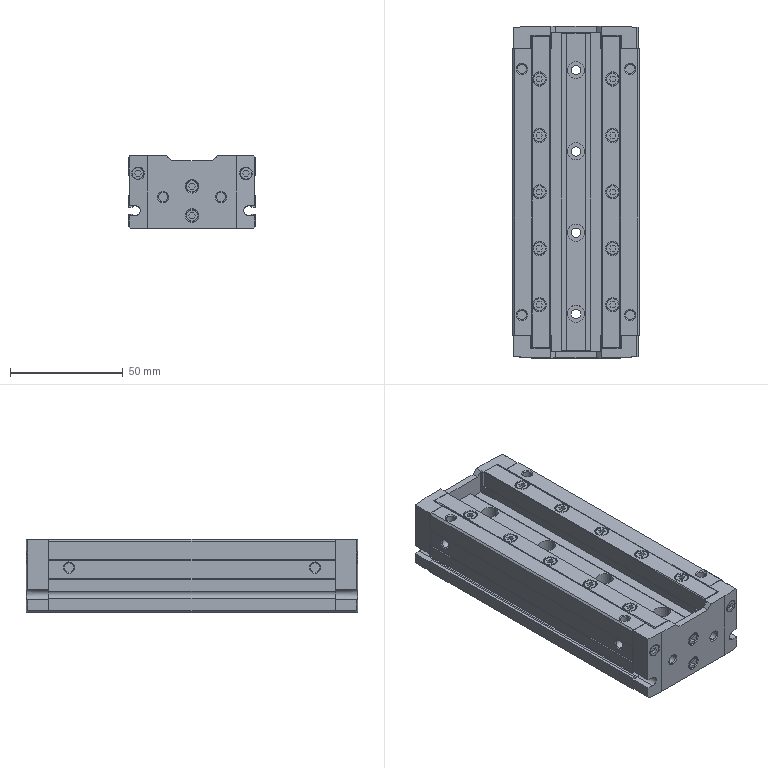Part | STEP file | 1 solid | 619 faces | box 56 x 147 x 32.5 mm | volume 222533 mm3 | plane 363 | cylinder 144 | cone 112 | commonest cylinder face diameters 5.5 x36 4.134 x28 6 x20 5.1 x16 3.7 x10 4.3 x10